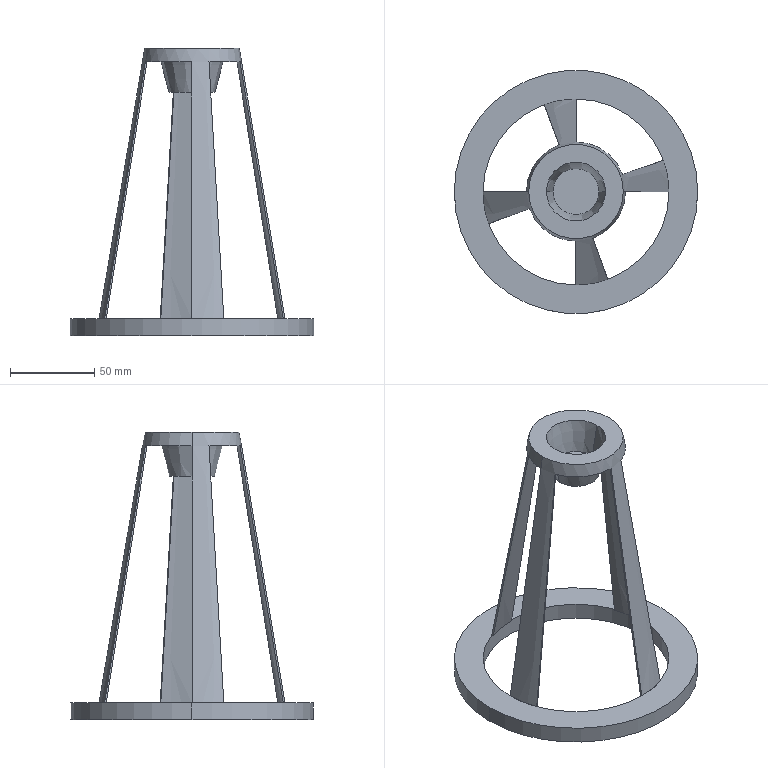Part | SolidWorks | features BaseBody 2 | 2 solids | 34 faces | box 144 x 144 x 170 mm | volume 89081 mm3 | plane 22 | cone 8 | cylinder 4 | commonest cylinder face diameters 110 x2 144 x2
STEP:
#1=CARTESIAN_POINT('',(55.,0.,0.));
#2=VERTEX_POINT('',#1);
#3=CARTESIAN_POINT('',(55.,0.,-10.));
#4=VERTEX_POINT('',#3);
#5=CARTESIAN_POINT('',(55.,0.,0.));
#6=DIRECTION('',(0.,0.,-1.));
#7=VECTOR('',#6,1000.);
#8=LINE('',#5,#7);
#9=EDGE_CURVE('',#2,#4,#8,.T.);
#10=ORIENTED_EDGE('',*,*,#9,.F.);
#11=CARTESIAN_POINT('',(-55.,0.,0.));
#12=VERTEX_POINT('',#11);
#13=CARTESIAN_POINT('',(0.,0.,0.));
#14=DIRECTION('',(0.,0.,-1.));
#15=DIRECTION('',(-1.,0.,0.));
#16=AXIS2_PLACEMENT_3D('',#13,#14,#15);
#17=CIRCLE('',#16,55.);
#18=EDGE_CURVE('',#12,#2,#17,.T.);
#19=ORIENTED_EDGE('',*,*,#18,.F.);
#20=CARTESIAN_POINT('',(-55.,0.,-10.));
#21=VERTEX_POINT('',#20);
#22=CARTESIAN_POINT('',(-55.,0.,0.));
#23=DIRECTION('',(0.,0.,-1.));
#24=VECTOR('',#23,1000.);
#25=LINE('',#22,#24);
#26=EDGE_CURVE('',#12,#21,#25,.T.);
#27=ORIENTED_EDGE('',*,*,#26,.T.);
#28=CARTESIAN_POINT('',(0.,0.,-10.));
#29=DIRECTION('',(0.,0.,-1.));
#30=DIRECTION('',(-1.,0.,0.));
#31=AXIS2_PLACEMENT_3D('',#28,#29,#30);
#32=CIRCLE('',#31,55.);
#33=EDGE_CURVE('',#21,#4,#32,.T.);
#34=ORIENTED_EDGE('',*,*,#33,.T.);
#35=EDGE_LOOP('',(#10,#19,#27,#34));
#36=FACE_OUTER_BOUND('',#35,.T.);
#37=CARTESIAN_POINT('',(0.,0.,0.));
#38=DIRECTION('',(0.,0.,-1.));
#39=DIRECTION('',(-1.,0.,0.));
#40=AXIS2_PLACEMENT_3D('',#37,#38,#39);
#41=CYLINDRICAL_SURFACE('',#40,55.);
#42=ADVANCED_FACE('',(#36),#41,.F.);
#43=ORIENTED_EDGE('',*,*,#33,.F.);
#44=CARTESIAN_POINT('',(0.,0.,-10.));
#45=DIRECTION('',(0.,0.,-1.));
#46=DIRECTION('',(-1.,0.,0.));
#47=AXIS2_PLACEMENT_3D('',#44,#45,#46);
#48=CIRCLE('',#47,55.);
#49=EDGE_CURVE('',#4,#21,#48,.T.);
#50=ORIENTED_EDGE('',*,*,#49,.F.);
#51=EDGE_LOOP('',(#43,#50));
#52=FACE_BOUND('',#51,.T.);
#53=CARTESIAN_POINT('',(72.,0.,-10.));
#54=VERTEX_POINT('',#53);
#55=CARTESIAN_POINT('',(-72.,0.,-10.));
#56=VERTEX_POINT('',#55);
#57=CARTESIAN_POINT('',(0.,0.,-10.));
#58=DIRECTION('',(0.,0.,-1.));
#59=DIRECTION('',(-1.,0.,0.));
#60=AXIS2_PLACEMENT_3D('',#57,#58,#59);
#61=CIRCLE('',#60,72.);
#62=EDGE_CURVE('',#54,#56,#61,.T.);
#63=ORIENTED_EDGE('',*,*,#62,.T.);
#64=CARTESIAN_POINT('',(0.,0.,-10.));
#65=DIRECTION('',(0.,0.,-1.));
#66=DIRECTION('',(-1.,0.,0.));
#67=AXIS2_PLACEMENT_3D('',#64,#65,#66);
#68=CIRCLE('',#67,72.);
#69=EDGE_CURVE('',#56,#54,#68,.T.);
#70=ORIENTED_EDGE('',*,*,#69,.T.);
#71=EDGE_LOOP('',(#63,#70));
#72=FACE_OUTER_BOUND('',#71,.T.);
#73=CARTESIAN_POINT('',(0.,0.,-10.));
#74=DIRECTION('',(0.,0.,-1.));
#75=DIRECTION('',(0.,-1.,0.));
#76=AXIS2_PLACEMENT_3D('',#73,#74,#75);
#77=PLANE('',#76);
#78=ADVANCED_FACE('',(#52,#72),#77,.T.);
#79=CARTESIAN_POINT('',(-72.,0.,0.));
#80=VERTEX_POINT('',#79);
#81=CARTESIAN_POINT('',(-72.,0.,-10.));
#82=DIRECTION('',(0.,0.,1.));
#83=VECTOR('',#82,1000.);
#84=LINE('',#81,#83);
#85=EDGE_CURVE('',#56,#80,#84,.T.);
#86=ORIENTED_EDGE('',*,*,#85,.F.);
#87=ORIENTED_EDGE('',*,*,#62,.F.);
#88=CARTESIAN_POINT('',(72.,0.,0.));
#89=VERTEX_POINT('',#88);
#90=CARTESIAN_POINT('',(72.,0.,-10.));
#91=DIRECTION('',(0.,0.,1.));
#92=VECTOR('',#91,1000.);
#93=LINE('',#90,#92);
#94=EDGE_CURVE('',#54,#89,#93,.T.);
#95=ORIENTED_EDGE('',*,*,#94,.T.);
#96=CARTESIAN_POINT('',(0.,0.,0.));
#97=DIRECTION('',(0.,0.,-1.));
#98=DIRECTION('',(-1.,0.,0.));
#99=AXIS2_PLACEMENT_3D('',#96,#97,#98);
#100=CIRCLE('',#99,72.);
#101=EDGE_CURVE('',#89,#80,#100,.T.);
#102=ORIENTED_EDGE('',*,*,#101,.T.);
#103=EDGE_LOOP('',(#86,#87,#95,#102));
#104=FACE_OUTER_BOUND('',#103,.T.);
#105=CARTESIAN_POINT('',(0.,0.,-10.));
#106=DIRECTION('',(0.,0.,1.));
#107=DIRECTION('',(1.,0.,0.));
#108=AXIS2_PLACEMENT_3D('',#105,#106,#107);
#109=CYLINDRICAL_SURFACE('',#108,72.);
#110=ADVANCED_FACE('',(#104),#109,.T.);
#111=ORIENTED_EDGE('',*,*,#18,.T.);
#112=CARTESIAN_POINT('',(0.,0.,0.));
#113=DIRECTION('',(0.,0.,-1.));
#114=DIRECTION('',(-1.,0.,0.));
#115=AXIS2_PLACEMENT_3D('',#112,#113,#114);
#116=CIRCLE('',#115,55.);
#117=EDGE_CURVE('',#2,#12,#116,.T.);
#118=ORIENTED_EDGE('',*,*,#117,.T.);
#119=EDGE_LOOP('',(#111,#118));
#120=FACE_BOUND('',#119,.T.);
#121=ORIENTED_EDGE('',*,*,#101,.F.);
#122=CARTESIAN_POINT('',(0.,0.,0.));
#123=DIRECTION('',(0.,0.,-1.));
#124=DIRECTION('',(-1.,0.,0.));
#125=AXIS2_PLACEMENT_3D('',#122,#123,#124);
#126=CIRCLE('',#125,72.);
#127=EDGE_CURVE('',#80,#89,#126,.T.);
#128=ORIENTED_EDGE('',*,*,#127,.F.);
#129=EDGE_LOOP('',(#121,#128));
#130=FACE_OUTER_BOUND('',#129,.T.);
#131=CARTESIAN_POINT('',(0.,0.,0.));
#132=DIRECTION('',(0.,0.,-1.));
#133=DIRECTION('',(0.,-1.,0.));
#134=AXIS2_PLACEMENT_3D('',#131,#132,#133);
#135=PLANE('',#134);
#136=ADVANCED_FACE('',(#120,#130),#135,.F.);
#137=ORIENTED_EDGE('',*,*,#69,.F.);
#138=ORIENTED_EDGE('',*,*,#85,.T.);
#139=ORIENTED_EDGE('',*,*,#127,.T.);
#140=ORIENTED_EDGE('',*,*,#94,.F.);
#141=EDGE_LOOP('',(#137,#138,#139,#140));
#142=FACE_OUTER_BOUND('',#141,.T.);
#143=CARTESIAN_POINT('',(0.,0.,-10.));
#144=DIRECTION('',(0.,0.,1.));
#145=DIRECTION('',(1.,0.,0.));
#146=AXIS2_PLACEMENT_3D('',#143,#144,#145);
#147=CYLINDRICAL_SURFACE('',#146,72.);
#148=ADVANCED_FACE('',(#142),#147,.T.);
#149=ORIENTED_EDGE('',*,*,#117,.F.);
#150=ORIENTED_EDGE('',*,*,#9,.T.);
#151=ORIENTED_EDGE('',*,*,#49,.T.);
#152=ORIENTED_EDGE('',*,*,#26,.F.);
#153=EDGE_LOOP('',(#149,#150,#151,#152));
#154=FACE_OUTER_BOUND('',#153,.T.);
#155=CARTESIAN_POINT('',(0.,0.,0.));
#156=DIRECTION('',(0.,0.,-1.));
#157=DIRECTION('',(-1.,0.,0.));
#158=AXIS2_PLACEMENT_3D('',#155,#156,#157);
#159=CYLINDRICAL_SURFACE('',#158,55.);
#160=ADVANCED_FACE('',(#154),#159,.F.);
#161=CLOSED_SHELL('',(#42,#78,#110,#136,#148,#160));
#162=MANIFOLD_SOLID_BREP('',#161);
#163=CARTESIAN_POINT('',(13.612,0.,140.));
#164=VERTEX_POINT('',#163);
#165=CARTESIAN_POINT('',(-13.612,0.,140.));
#166=VERTEX_POINT('',#165);
#167=CARTESIAN_POINT('',(0.,0.,140.));
#168=DIRECTION('',(0.,0.,1.));
#169=DIRECTION('',(1.,0.,0.));
#170=AXIS2_PLACEMENT_3D('',#167,#168,#169);
#171=CIRCLE('',#170,13.612);
#172=EDGE_CURVE('',#164,#166,#171,.T.);
#173=ORIENTED_EDGE('',*,*,#172,.T.);
#174=CARTESIAN_POINT('',(0.,0.,140.));
#175=DIRECTION('',(0.,0.,1.));
#176=DIRECTION('',(1.,0.,0.));
#177=AXIS2_PLACEMENT_3D('',#174,#175,#176);
#178=CIRCLE('',#177,13.612);
#179=EDGE_CURVE('',#166,#164,#178,.T.);
#180=ORIENTED_EDGE('',*,*,#179,.T.);
#181=EDGE_LOOP('',(#173,#180));
#182=FACE_OUTER_BOUND('',#181,.T.);
#183=CARTESIAN_POINT('',(0.,0.,140.));
#184=DIRECTION('',(0.,0.,1.));
#185=DIRECTION('',(1.,0.,0.));
#186=AXIS2_PLACEMENT_3D('',#183,#184,#185);
#187=PLANE('',#186);
#188=ADVANCED_FACE('',(#182),#187,.T.);
#189=CARTESIAN_POINT('',(-17.5,0.,160.));
#190=VERTEX_POINT('',#189);
#191=CARTESIAN_POINT('',(-17.5,0.,160.));
#192=DIRECTION('',(-0.1908,0.,0.9816));
#193=VECTOR('',#192,1000.);
#194=LINE('',#191,#193);
#195=EDGE_CURVE('',#166,#190,#194,.T.);
#196=ORIENTED_EDGE('',*,*,#195,.F.);
#197=ORIENTED_EDGE('',*,*,#172,.F.);
#198=CARTESIAN_POINT('',(17.5,0.,160.));
#199=VERTEX_POINT('',#198);
#200=CARTESIAN_POINT('',(17.5,0.,160.));
#201=DIRECTION('',(0.1908,0.,0.9816));
#202=VECTOR('',#201,1000.);
#203=LINE('',#200,#202);
#204=EDGE_CURVE('',#164,#199,#203,.T.);
#205=ORIENTED_EDGE('',*,*,#204,.T.);
#206=CARTESIAN_POINT('',(0.,0.,160.));
#207=DIRECTION('',(0.,0.,1.));
#208=DIRECTION('',(1.,0.,0.));
#209=AXIS2_PLACEMENT_3D('',#206,#207,#208);
#210=CIRCLE('',#209,17.5);
#211=EDGE_CURVE('',#199,#190,#210,.T.);
#212=ORIENTED_EDGE('',*,*,#211,.T.);
#213=EDGE_LOOP('',(#196,#197,#205,#212));
#214=FACE_OUTER_BOUND('',#213,.T.);
#215=CARTESIAN_POINT('',(0.,0.,160.));
#216=DIRECTION('',(0.,0.,1.));
#217=DIRECTION('',(1.,0.,0.));
#218=AXIS2_PLACEMENT_3D('',#215,#216,#217);
#219=CONICAL_SURFACE('',#218,17.5,0.192);
#220=ADVANCED_FACE('',(#214),#219,.F.);
#221=CARTESIAN_POINT('',(-13.569,0.,134.));
#222=VERTEX_POINT('',#221);
#223=CARTESIAN_POINT('',(13.569,0.,134.));
#224=VERTEX_POINT('',#223);
#225=CARTESIAN_POINT('',(0.,0.,134.));
#226=DIRECTION('',(0.,0.,-1.));
#227=DIRECTION('',(-1.,0.,0.));
#228=AXIS2_PLACEMENT_3D('',#225,#226,#227);
#229=CIRCLE('',#228,13.569);
#230=EDGE_CURVE('',#222,#224,#229,.T.);
#231=ORIENTED_EDGE('',*,*,#230,.T.);
#232=CARTESIAN_POINT('',(0.,0.,134.));
#233=DIRECTION('',(0.,0.,-1.));
#234=DIRECTION('',(-1.,0.,0.));
#235=AXIS2_PLACEMENT_3D('',#232,#233,#234);
#236=CIRCLE('',#235,13.569);
#237=EDGE_CURVE('',#224,#222,#236,.T.);
#238=ORIENTED_EDGE('',*,*,#237,.T.);
#239=EDGE_LOOP('',(#231,#238));
#240=FACE_OUTER_BOUND('',#239,.T.);
#241=CARTESIAN_POINT('',(0.,0.,134.));
#242=DIRECTION('',(0.,0.,-1.));
#243=DIRECTION('',(0.,-1.,0.));
#244=AXIS2_PLACEMENT_3D('',#241,#242,#243);
#245=PLANE('',#244);
#246=ADVANCED_FACE('',(#240),#245,.T.);
#247=CARTESIAN_POINT('',(20.,0.,158.));
#248=VERTEX_POINT('',#247);
#249=CARTESIAN_POINT('',(20.,0.,158.));
#250=DIRECTION('',(0.2588,0.,0.9659));
#251=VECTOR('',#250,1000.);
#252=LINE('',#249,#251);
#253=EDGE_CURVE('',#224,#248,#252,.T.);
#254=ORIENTED_EDGE('',*,*,#253,.F.);
#255=ORIENTED_EDGE('',*,*,#230,.F.);
#256=CARTESIAN_POINT('',(-20.,0.,158.));
#257=VERTEX_POINT('',#256);
#258=CARTESIAN_POINT('',(-20.,0.,158.));
#259=DIRECTION('',(-0.2588,0.,0.9659));
#260=VECTOR('',#259,1000.);
#261=LINE('',#258,#260);
#262=EDGE_CURVE('',#222,#257,#261,.T.);
#263=ORIENTED_EDGE('',*,*,#262,.T.);
#264=CARTESIAN_POINT('',(0.,0.,158.));
#265=DIRECTION('',(0.,0.,-1.));
#266=DIRECTION('',(1.,0.,0.));
#267=AXIS2_PLACEMENT_3D('',#264,#265,#266);
#268=CIRCLE('',#267,20.);
#269=EDGE_CURVE('',#257,#248,#268,.T.);
#270=ORIENTED_EDGE('',*,*,#269,.T.);
#271=EDGE_LOOP('',(#254,#255,#263,#270));
#272=FACE_OUTER_BOUND('',#271,.T.);
#273=CARTESIAN_POINT('',(0.,0.,158.));
#274=DIRECTION('',(0.,0.,1.));
#275=DIRECTION('',(-1.,0.,0.));
#276=AXIS2_PLACEMENT_3D('',#273,#274,#275);
#277=CONICAL_SURFACE('',#276,20.,0.2618);
#278=ADVANCED_FACE('',(#272),#277,.T.);
#279=CARTESIAN_POINT('',(0.,-28.336,152.));
#280=VERTEX_POINT('',#279);
#281=CARTESIAN_POINT('',(0.,-53.986,0.));
#282=VERTEX_POINT('',#281);
#283=CARTESIAN_POINT('',(0.,0.,319.916));
#284=DIRECTION('',(0.,-0.1664,-0.9861));
#285=VECTOR('',#284,1000.);
#286=LINE('',#283,#285);
#287=EDGE_CURVE('',#280,#282,#286,.T.);
#288=ORIENTED_EDGE('',*,*,#287,.T.);
#289=CARTESIAN_POINT('',(0.,-55.,0.));
#290=VERTEX_POINT('',#289);
#291=CARTESIAN_POINT('',(0.,-49.,0.));
#292=DIRECTION('',(0.,-1.,0.));
#293=VECTOR('',#292,1000.);
#294=LINE('',#291,#293);
#295=EDGE_CURVE('',#282,#290,#294,.T.);
#296=ORIENTED_EDGE('',*,*,#295,.T.);
#297=CARTESIAN_POINT('',(0.,-29.35,152.));
#298=VERTEX_POINT('',#297);
#299=CARTESIAN_POINT('',(0.,-55.,0.));
#300=DIRECTION('',(0.,0.1664,0.9861));
#301=VECTOR('',#300,1000.);
#302=LINE('',#299,#301);
#303=EDGE_CURVE('',#290,#298,#302,.T.);
#304=ORIENTED_EDGE('',*,*,#303,.T.);
#305=CARTESIAN_POINT('',(0.,-29.35,152.));
#306=DIRECTION('',(0.,1.,0.));
#307=VECTOR('',#306,1000.);
#308=LINE('',#305,#307);
#309=EDGE_CURVE('',#298,#280,#308,.T.);
#310=ORIENTED_EDGE('',*,*,#309,.T.);
#311=EDGE_LOOP('',(#288,#296,#304,#310));
#312=FACE_OUTER_BOUND('',#311,.T.);
#313=CARTESIAN_POINT('',(0.,0.,0.));
#314=DIRECTION('',(-1.,0.,0.));
#315=DIRECTION('',(0.,0.,1.));
#316=AXIS2_PLACEMENT_3D('',#313,#314,#315);
#317=PLANE('',#316);
#318=ADVANCED_FACE('',(#312),#317,.T.);
#319=CARTESIAN_POINT('',(-27.58,-10.038,152.));
#320=VERTEX_POINT('',#319);
#321=CARTESIAN_POINT('',(-26.627,-9.691,152.));
#322=VERTEX_POINT('',#321);
#323=CARTESIAN_POINT('',(-27.58,-10.038,152.));
#324=DIRECTION('',(0.9397,0.342,0.));
#325=VECTOR('',#324,1000.);
#326=LINE('',#323,#325);
#327=EDGE_CURVE('',#320,#322,#326,.T.);
#328=ORIENTED_EDGE('',*,*,#327,.F.);
#329=CARTESIAN_POINT('',(-51.683,-18.811,0.));
#330=VERTEX_POINT('',#329);
#331=CARTESIAN_POINT('',(-51.683,-18.811,0.));
#332=DIRECTION('',(0.1564,0.05691,0.9861));
#333=VECTOR('',#332,1000.);
#334=LINE('',#331,#333);
#335=EDGE_CURVE('',#330,#320,#334,.T.);
#336=ORIENTED_EDGE('',*,*,#335,.F.);
#337=CARTESIAN_POINT('',(-50.73,-18.464,0.));
#338=VERTEX_POINT('',#337);
#339=CARTESIAN_POINT('',(-46.045,-16.759,0.));
#340=DIRECTION('',(-0.9397,-0.342,0.));
#341=VECTOR('',#340,1000.);
#342=LINE('',#339,#341);
#343=EDGE_CURVE('',#338,#330,#342,.T.);
#344=ORIENTED_EDGE('',*,*,#343,.F.);
#345=CARTESIAN_POINT('',(0.,0.,319.916));
#346=DIRECTION('',(-0.1564,-0.05691,-0.9861));
#347=VECTOR('',#346,1000.);
#348=LINE('',#345,#347);
#349=EDGE_CURVE('',#322,#338,#348,.T.);
#350=ORIENTED_EDGE('',*,*,#349,.F.);
#351=EDGE_LOOP('',(#328,#336,#344,#350));
#352=FACE_OUTER_BOUND('',#351,.T.);
#353=CARTESIAN_POINT('',(0.,0.,0.));
#354=DIRECTION('',(-0.342,0.9397,0.));
#355=DIRECTION('',(0.,0.,1.));
#356=AXIS2_PLACEMENT_3D('',#353,#354,#355);
#357=PLANE('',#356);
#358=ADVANCED_FACE('',(#352),#357,.F.);
#359=CARTESIAN_POINT('',(0.,0.,152.));
#360=DIRECTION('',(0.,0.,1.));
#361=DIRECTION('',(-1.,0.,0.));
#362=AXIS2_PLACEMENT_3D('',#359,#360,#361);
#363=CIRCLE('',#362,28.336);
#364=EDGE_CURVE('',#322,#280,#363,.T.);
#365=ORIENTED_EDGE('',*,*,#364,.T.);
#366=ORIENTED_EDGE('',*,*,#309,.F.);
#367=CARTESIAN_POINT('',(0.,0.,152.));
#368=DIRECTION('',(0.,0.,1.));
#369=DIRECTION('',(0.,1.,0.));
#370=AXIS2_PLACEMENT_3D('',#367,#368,#369);
#371=CIRCLE('',#370,29.35);
#372=EDGE_CURVE('',#320,#298,#371,.T.);
#373=ORIENTED_EDGE('',*,*,#372,.F.);
#374=ORIENTED_EDGE('',*,*,#327,.T.);
#375=EDGE_LOOP('',(#365,#366,#373,#374));
#376=FACE_OUTER_BOUND('',#375,.T.);
#377=CARTESIAN_POINT('',(-27.58,-10.038,152.));
#378=DIRECTION('',(0.,0.,-1.));
#379=DIRECTION('',(0.,-1.,0.));
#380=AXIS2_PLACEMENT_3D('',#377,#378,#379);
#381=PLANE('',#380);
#382=ADVANCED_FACE('',(#376),#381,.T.);
#383=CARTESIAN_POINT('',(28.336,0.,152.));
#384=VERTEX_POINT('',#383);
#385=CARTESIAN_POINT('',(53.986,0.,0.));
#386=VERTEX_POINT('',#385);
#387=CARTESIAN_POINT('',(0.,0.,319.916));
#388=DIRECTION('',(0.1664,0.,-0.9861));
#389=VECTOR('',#388,1000.);
#390=LINE('',#387,#389);
#391=EDGE_CURVE('',#384,#386,#390,.T.);
#392=ORIENTED_EDGE('',*,*,#391,.T.);
#393=CARTESIAN_POINT('',(55.,0.,0.));
#394=VERTEX_POINT('',#393);
#395=CARTESIAN_POINT('',(49.,0.,0.));
#396=DIRECTION('',(1.,0.,0.));
#397=VECTOR('',#396,1000.);
#398=LINE('',#395,#397);
#399=EDGE_CURVE('',#386,#394,#398,.T.);
#400=ORIENTED_EDGE('',*,*,#399,.T.);
#401=CARTESIAN_POINT('',(29.35,0.,152.));
#402=VERTEX_POINT('',#401);
#403=CARTESIAN_POINT('',(55.,0.,0.));
#404=DIRECTION('',(-0.1664,0.,0.9861));
#405=VECTOR('',#404,1000.);
#406=LINE('',#403,#405);
#407=EDGE_CURVE('',#394,#402,#406,.T.);
#408=ORIENTED_EDGE('',*,*,#407,.T.);
#409=CARTESIAN_POINT('',(29.35,0.,152.));
#410=DIRECTION('',(-1.,0.,0.));
#411=VECTOR('',#410,1000.);
#412=LINE('',#409,#411);
#413=EDGE_CURVE('',#402,#384,#412,.T.);
#414=ORIENTED_EDGE('',*,*,#413,.T.);
#415=EDGE_LOOP('',(#392,#400,#408,#414));
#416=FACE_OUTER_BOUND('',#415,.T.);
#417=CARTESIAN_POINT('',(0.,0.,0.));
#418=DIRECTION('',(0.,-1.,0.));
#419=DIRECTION('',(0.,0.,-1.));
#420=AXIS2_PLACEMENT_3D('',#417,#418,#419);
#421=PLANE('',#420);
#422=ADVANCED_FACE('',(#416),#421,.T.);
#423=CARTESIAN_POINT('',(10.038,-27.58,152.));
#424=VERTEX_POINT('',#423);
#425=CARTESIAN_POINT('',(9.691,-26.627,152.));
#426=VERTEX_POINT('',#425);
#427=CARTESIAN_POINT('',(10.038,-27.58,152.));
#428=DIRECTION('',(-0.342,0.9397,0.));
#429=VECTOR('',#428,1000.);
#430=LINE('',#427,#429);
#431=EDGE_CURVE('',#424,#426,#430,.T.);
#432=ORIENTED_EDGE('',*,*,#431,.F.);
#433=CARTESIAN_POINT('',(18.811,-51.683,0.));
#434=VERTEX_POINT('',#433);
#435=CARTESIAN_POINT('',(18.811,-51.683,0.));
#436=DIRECTION('',(-0.05691,0.1564,0.9861));
#437=VECTOR('',#436,1000.);
#438=LINE('',#435,#437);
#439=EDGE_CURVE('',#434,#424,#438,.T.);
#440=ORIENTED_EDGE('',*,*,#439,.F.);
#441=CARTESIAN_POINT('',(18.464,-50.73,0.));
#442=VERTEX_POINT('',#441);
#443=CARTESIAN_POINT('',(16.759,-46.045,0.));
#444=DIRECTION('',(0.342,-0.9397,0.));
#445=VECTOR('',#444,1000.);
#446=LINE('',#443,#445);
#447=EDGE_CURVE('',#442,#434,#446,.T.);
#448=ORIENTED_EDGE('',*,*,#447,.F.);
#449=CARTESIAN_POINT('',(0.,0.,319.916));
#450=DIRECTION('',(0.05691,-0.1564,-0.9861));
#451=VECTOR('',#450,1000.);
#452=LINE('',#449,#451);
#453=EDGE_CURVE('',#426,#442,#452,.T.);
#454=ORIENTED_EDGE('',*,*,#453,.F.);
#455=EDGE_LOOP('',(#432,#440,#448,#454));
#456=FACE_OUTER_BOUND('',#455,.T.);
#457=CARTESIAN_POINT('',(0.,0.,0.));
#458=DIRECTION('',(-0.9397,-0.342,0.));
#459=DIRECTION('',(-0.342,0.9397,0.));
#460=AXIS2_PLACEMENT_3D('',#457,#458,#459);
#461=PLANE('',#460);
#462=ADVANCED_FACE('',(#456),#461,.F.);
#463=CARTESIAN_POINT('',(0.,0.,152.));
#464=DIRECTION('',(0.,0.,1.));
#465=DIRECTION('',(-1.,0.,0.));
#466=AXIS2_PLACEMENT_3D('',#463,#464,#465);
#467=CIRCLE('',#466,28.336);
#468=EDGE_CURVE('',#426,#384,#467,.T.);
#469=ORIENTED_EDGE('',*,*,#468,.T.);
#470=ORIENTED_EDGE('',*,*,#413,.F.);
#471=CARTESIAN_POINT('',(0.,0.,152.));
#472=DIRECTION('',(0.,0.,1.));
#473=DIRECTION('',(-1.,0.,0.));
#474=AXIS2_PLACEMENT_3D('',#471,#472,#473);
#475=CIRCLE('',#474,29.35);
#476=EDGE_CURVE('',#424,#402,#475,.T.);
#477=ORIENTED_EDGE('',*,*,#476,.F.);
#478=ORIENTED_EDGE('',*,*,#431,.T.);
#479=EDGE_LOOP('',(#469,#470,#477,#478));
#480=FACE_OUTER_BOUND('',#479,.T.);
#481=CARTESIAN_POINT('',(10.038,-27.58,152.));
#482=DIRECTION('',(0.,0.,-1.));
#483=DIRECTION('',(0.,-1.,0.));
#484=AXIS2_PLACEMENT_3D('',#481,#482,#483);
#485=PLANE('',#484);
#486=ADVANCED_FACE('',(#480),#485,.T.);
#487=CARTESIAN_POINT('',(0.,28.336,152.));
#488=VERTEX_POINT('',#487);
#489=CARTESIAN_POINT('',(0.,53.986,0.));
#490=VERTEX_POINT('',#489);
#491=CARTESIAN_POINT('',(0.,0.,319.916));
#492=DIRECTION('',(0.,0.1664,-0.9861));
#493=VECTOR('',#492,1000.);
#494=LINE('',#491,#493);
#495=EDGE_CURVE('',#488,#490,#494,.T.);
#496=ORIENTED_EDGE('',*,*,#495,.T.);
#497=CARTESIAN_POINT('',(0.,55.,0.));
#498=VERTEX_POINT('',#497);
#499=CARTESIAN_POINT('',(0.,49.,0.));
#500=DIRECTION('',(0.,1.,0.));
#501=VECTOR('',#500,1000.);
#502=LINE('',#499,#501);
#503=EDGE_CURVE('',#490,#498,#502,.T.);
#504=ORIENTED_EDGE('',*,*,#503,.T.);
#505=CARTESIAN_POINT('',(0.,29.35,152.));
#506=VERTEX_POINT('',#505);
#507=CARTESIAN_POINT('',(0.,55.,0.));
#508=DIRECTION('',(0.,-0.1664,0.9861));
#509=VECTOR('',#508,1000.);
#510=LINE('',#507,#509);
#511=EDGE_CURVE('',#498,#506,#510,.T.);
#512=ORIENTED_EDGE('',*,*,#511,.T.);
#513=CARTESIAN_POINT('',(0.,29.35,152.));
#514=DIRECTION('',(0.,-1.,0.));
#515=VECTOR('',#514,1000.);
#516=LINE('',#513,#515);
#517=EDGE_CURVE('',#506,#488,#516,.T.);
#518=ORIENTED_EDGE('',*,*,#517,.T.);
#519=EDGE_LOOP('',(#496,#504,#512,#518));
#520=FACE_OUTER_BOUND('',#519,.T.);
#521=CARTESIAN_POINT('',(0.,0.,0.));
#522=DIRECTION('',(1.,0.,0.));
#523=DIRECTION('',(0.,-1.,0.));
#524=AXIS2_PLACEMENT_3D('',#521,#522,#523);
#525=PLANE('',#524);
#526=ADVANCED_FACE('',(#520),#525,.T.);
#527=CARTESIAN_POINT('',(27.58,10.038,152.));
#528=VERTEX_POINT('',#527);
#529=CARTESIAN_POINT('',(26.627,9.691,152.));
#530=VERTEX_POINT('',#529);
#531=CARTESIAN_POINT('',(27.58,10.038,152.));
#532=DIRECTION('',(-0.9397,-0.342,0.));
#533=VECTOR('',#532,1000.);
#534=LINE('',#531,#533);
#535=EDGE_CURVE('',#528,#530,#534,.T.);
#536=ORIENTED_EDGE('',*,*,#535,.F.);
#537=CARTESIAN_POINT('',(51.683,18.811,0.));
#538=VERTEX_POINT('',#537);
#539=CARTESIAN_POINT('',(51.683,18.811,0.));
#540=DIRECTION('',(-0.1564,-0.05691,0.9861));
#541=VECTOR('',#540,1000.);
#542=LINE('',#539,#541);
#543=EDGE_CURVE('',#538,#528,#542,.T.);
#544=ORIENTED_EDGE('',*,*,#543,.F.);
#545=CARTESIAN_POINT('',(50.73,18.464,0.));
#546=VERTEX_POINT('',#545);
#547=CARTESIAN_POINT('',(46.045,16.759,0.));
#548=DIRECTION('',(0.9397,0.342,0.));
#549=VECTOR('',#548,1000.);
#550=LINE('',#547,#549);
#551=EDGE_CURVE('',#546,#538,#550,.T.);
#552=ORIENTED_EDGE('',*,*,#551,.F.);
#553=CARTESIAN_POINT('',(0.,0.,319.916));
#554=DIRECTION('',(0.1564,0.05691,-0.9861));
#555=VECTOR('',#554,1000.);
#556=LINE('',#553,#555);
#557=EDGE_CURVE('',#530,#546,#556,.T.);
#558=ORIENTED_EDGE('',*,*,#557,.F.);
#559=EDGE_LOOP('',(#536,#544,#552,#558));
#560=FACE_OUTER_BOUND('',#559,.T.);
#561=CARTESIAN_POINT('',(0.,0.,0.));
#562=DIRECTION('',(0.342,-0.9397,0.));
#563=DIRECTION('',(0.,0.,-1.));
#564=AXIS2_PLACEMENT_3D('',#561,#562,#563);
#565=PLANE('',#564);
#566=ADVANCED_FACE('',(#560),#565,.F.);
#567=CARTESIAN_POINT('',(0.,0.,152.));
#568=DIRECTION('',(0.,0.,1.));
#569=DIRECTION('',(-1.,0.,0.));
#570=AXIS2_PLACEMENT_3D('',#567,#568,#569);
#571=CIRCLE('',#570,28.336);
#572=EDGE_CURVE('',#530,#488,#571,.T.);
#573=ORIENTED_EDGE('',*,*,#572,.T.);
#574=ORIENTED_EDGE('',*,*,#517,.F.);
#575=CARTESIAN_POINT('',(0.,0.,152.));
#576=DIRECTION('',(0.,0.,1.));
#577=DIRECTION('',(0.,-1.,0.));
#578=AXIS2_PLACEMENT_3D('',#575,#576,#577);
#579=CIRCLE('',#578,29.35);
#580=EDGE_CURVE('',#528,#506,#579,.T.);
#581=ORIENTED_EDGE('',*,*,#580,.F.);
#582=ORIENTED_EDGE('',*,*,#535,.T.);
#583=EDGE_LOOP('',(#573,#574,#581,#582));
#584=FACE_OUTER_BOUND('',#583,.T.);
#585=CARTESIAN_POINT('',(27.58,10.038,152.));
#586=DIRECTION('',(0.,0.,-1.));
#587=DIRECTION('',(0.,-1.,0.));
#588=AXIS2_PLACEMENT_3D('',#585,#586,#587);
#589=PLANE('',#588);
#590=ADVANCED_FACE('',(#584),#589,.T.);
#591=CARTESIAN_POINT('',(-28.336,0.,152.));
#592=VERTEX_POINT('',#591);
#593=CARTESIAN_POINT('',(-53.986,0.,0.));
#594=VERTEX_POINT('',#593);
#595=CARTESIAN_POINT('',(0.,0.,319.916));
#596=DIRECTION('',(-0.1664,0.,-0.9861));
#597=VECTOR('',#596,1000.);
#598=LINE('',#595,#597);
#599=EDGE_CURVE('',#592,#594,#598,.T.);
#600=ORIENTED_EDGE('',*,*,#599,.T.);
#601=CARTESIAN_POINT('',(-55.,0.,0.));
#602=VERTEX_POINT('',#601);
#603=CARTESIAN_POINT('',(-49.,0.,0.));
#604=DIRECTION('',(-1.,0.,0.));
#605=VECTOR('',#604,1000.);
#606=LINE('',#603,#605);
#607=EDGE_CURVE('',#594,#602,#606,.T.);
#608=ORIENTED_EDGE('',*,*,#607,.T.);
#609=CARTESIAN_POINT('',(-29.35,0.,152.));
#610=VERTEX_POINT('',#609);
#611=CARTESIAN_POINT('',(-55.,0.,0.));
#612=DIRECTION('',(0.1664,0.,0.9861));
#613=VECTOR('',#612,1000.);
#614=LINE('',#611,#613);
#615=EDGE_CURVE('',#602,#610,#614,.T.);
#616=ORIENTED_EDGE('',*,*,#615,.T.);
#617=CARTESIAN_POINT('',(-29.35,0.,152.));
#618=DIRECTION('',(1.,0.,0.));
#619=VECTOR('',#618,1000.);
#620=LINE('',#617,#619);
#621=EDGE_CURVE('',#610,#592,#620,.T.);
#622=ORIENTED_EDGE('',*,*,#621,.T.);
#623=EDGE_LOOP('',(#600,#608,#616,#622));
#624=FACE_OUTER_BOUND('',#623,.T.);
#625=CARTESIAN_POINT('',(0.,0.,0.));
#626=DIRECTION('',(0.,1.,0.));
#627=DIRECTION('',(1.,0.,0.));
#628=AXIS2_PLACEMENT_3D('',#625,#626,#627);
#629=PLANE('',#628);
#630=ADVANCED_FACE('',(#624),#629,.T.);
#631=CARTESIAN_POINT('',(-10.038,27.58,152.));
#632=VERTEX_POINT('',#631);
#633=CARTESIAN_POINT('',(-9.691,26.627,152.));
#634=VERTEX_POINT('',#633);
#635=CARTESIAN_POINT('',(-10.038,27.58,152.));
#636=DIRECTION('',(0.342,-0.9397,0.));
#637=VECTOR('',#636,1000.);
#638=LINE('',#635,#637);
#639=EDGE_CURVE('',#632,#634,#638,.T.);
#640=ORIENTED_EDGE('',*,*,#639,.F.);
#641=CARTESIAN_POINT('',(-18.811,51.683,0.));
#642=VERTEX_POINT('',#641);
#643=CARTESIAN_POINT('',(-18.811,51.683,0.));
#644=DIRECTION('',(0.05691,-0.1564,0.9861));
#645=VECTOR('',#644,1000.);
#646=LINE('',#643,#645);
#647=EDGE_CURVE('',#642,#632,#646,.T.);
#648=ORIENTED_EDGE('',*,*,#647,.F.);
#649=CARTESIAN_POINT('',(-18.464,50.73,0.));
#650=VERTEX_POINT('',#649);
#651=CARTESIAN_POINT('',(-16.759,46.045,0.));
#652=DIRECTION('',(-0.342,0.9397,0.));
#653=VECTOR('',#652,1000.);
#654=LINE('',#651,#653);
#655=EDGE_CURVE('',#650,#642,#654,.T.);
#656=ORIENTED_EDGE('',*,*,#655,.F.);
#657=CARTESIAN_POINT('',(0.,0.,319.916));
#658=DIRECTION('',(-0.05691,0.1564,-0.9861));
#659=VECTOR('',#658,1000.);
#660=LINE('',#657,#659);
#661=EDGE_CURVE('',#634,#650,#660,.T.);
#662=ORIENTED_EDGE('',*,*,#661,.F.);
#663=EDGE_LOOP('',(#640,#648,#656,#662));
#664=FACE_OUTER_BOUND('',#663,.T.);
#665=CARTESIAN_POINT('',(0.,0.,0.));
#666=DIRECTION('',(0.9397,0.342,0.));
#667=DIRECTION('',(0.,0.,-1.));
#668=AXIS2_PLACEMENT_3D('',#665,#666,#667);
#669=PLANE('',#668);
#670=ADVANCED_FACE('',(#664),#669,.F.);
#671=CARTESIAN_POINT('',(0.,0.,152.));
#672=DIRECTION('',(0.,0.,1.));
#673=DIRECTION('',(-1.,0.,0.));
#674=AXIS2_PLACEMENT_3D('',#671,#672,#673);
#675=CIRCLE('',#674,28.336);
#676=EDGE_CURVE('',#634,#592,#675,.T.);
#677=ORIENTED_EDGE('',*,*,#676,.T.);
#678=ORIENTED_EDGE('',*,*,#621,.F.);
#679=CARTESIAN_POINT('',(0.,0.,152.));
#680=DIRECTION('',(0.,0.,1.));
#681=DIRECTION('',(1.,0.,0.));
#682=AXIS2_PLACEMENT_3D('',#679,#680,#681);
#683=CIRCLE('',#682,29.35);
#684=EDGE_CURVE('',#632,#610,#683,.T.);
#685=ORIENTED_EDGE('',*,*,#684,.F.);
#686=ORIENTED_EDGE('',*,*,#639,.T.);
#687=EDGE_LOOP('',(#677,#678,#685,#686));
#688=FACE_OUTER_BOUND('',#687,.T.);
#689=CARTESIAN_POINT('',(-10.038,27.58,152.));
#690=DIRECTION('',(0.,0.,-1.));
#691=DIRECTION('',(0.,-1.,0.));
#692=AXIS2_PLACEMENT_3D('',#689,#690,#691);
#693=PLANE('',#692);
#694=ADVANCED_FACE('',(#688),#693,.T.);
#695=CARTESIAN_POINT('',(28.,0.,160.));
#696=VERTEX_POINT('',#695);
#697=CARTESIAN_POINT('',(28.,0.,160.));
#698=DIRECTION('',(0.1664,0.,-0.9861));
#699=VECTOR('',#698,1000.);
#700=LINE('',#697,#699);
#701=EDGE_CURVE('',#696,#402,#700,.T.);
#702=ORIENTED_EDGE('',*,*,#701,.F.);
#703=CARTESIAN_POINT('',(-28.,0.,160.));
#704=VERTEX_POINT('',#703);
#705=CARTESIAN_POINT('',(0.,0.,160.));
#706=DIRECTION('',(0.,0.,1.));
#707=DIRECTION('',(1.,0.,0.));
#708=AXIS2_PLACEMENT_3D('',#705,#706,#707);
#709=CIRCLE('',#708,28.);
#710=EDGE_CURVE('',#704,#696,#709,.T.);
#711=ORIENTED_EDGE('',*,*,#710,.F.);
#712=CARTESIAN_POINT('',(-28.,0.,160.));
#713=DIRECTION('',(-0.1664,0.,-0.9861));
#714=VECTOR('',#713,1000.);
#715=LINE('',#712,#714);
#716=EDGE_CURVE('',#704,#610,#715,.T.);
#717=ORIENTED_EDGE('',*,*,#716,.T.);
#718=ORIENTED_EDGE('',*,*,#615,.F.);
#719=CARTESIAN_POINT('',(0.,0.,0.));
#720=DIRECTION('',(0.,0.,-1.));
#721=DIRECTION('',(-1.,0.,0.));
#722=AXIS2_PLACEMENT_3D('',#719,#720,#721);
#723=CIRCLE('',#722,55.);
#724=EDGE_CURVE('',#330,#602,#723,.T.);
#725=ORIENTED_EDGE('',*,*,#724,.F.);
#726=ORIENTED_EDGE('',*,*,#335,.T.);
#727=ORIENTED_EDGE('',*,*,#372,.T.);
#728=ORIENTED_EDGE('',*,*,#303,.F.);
#729=CARTESIAN_POINT('',(0.,0.,0.));
#730=DIRECTION('',(0.,0.,-1.));
#731=DIRECTION('',(-1.,0.,0.));
#732=AXIS2_PLACEMENT_3D('',#729,#730,#731);
#733=CIRCLE('',#732,55.);
#734=EDGE_CURVE('',#434,#290,#733,.T.);
#735=ORIENTED_EDGE('',*,*,#734,.F.);
#736=ORIENTED_EDGE('',*,*,#439,.T.);
#737=ORIENTED_EDGE('',*,*,#476,.T.);
#738=EDGE_LOOP('',(#702,#711,#717,#718,#725,#726,#727,#728,#735,#736,#737));
#739=FACE_OUTER_BOUND('',#738,.T.);
#740=CARTESIAN_POINT('',(0.,0.,160.));
#741=DIRECTION('',(0.,0.,-1.));
#742=DIRECTION('',(-1.,0.,0.));
#743=AXIS2_PLACEMENT_3D('',#740,#741,#742);
#744=CONICAL_SURFACE('',#743,28.,0.1672);
#745=ADVANCED_FACE('',(#739),#744,.T.);
#746=ORIENTED_EDGE('',*,*,#211,.F.);
#747=CARTESIAN_POINT('',(0.,0.,160.));
#748=DIRECTION('',(0.,0.,1.));
#749=DIRECTION('',(1.,0.,0.));
#750=AXIS2_PLACEMENT_3D('',#747,#748,#749);
#751=CIRCLE('',#750,17.5);
#752=EDGE_CURVE('',#190,#199,#751,.T.);
#753=ORIENTED_EDGE('',*,*,#752,.F.);
#754=EDGE_LOOP('',(#746,#753));
#755=FACE_BOUND('',#754,.T.);
#756=ORIENTED_EDGE('',*,*,#710,.T.);
#757=CARTESIAN_POINT('',(0.,0.,160.));
#758=DIRECTION('',(0.,0.,1.));
#759=DIRECTION('',(1.,0.,0.));
#760=AXIS2_PLACEMENT_3D('',#757,#758,#759);
#761=CIRCLE('',#760,28.);
#762=EDGE_CURVE('',#696,#704,#761,.T.);
#763=ORIENTED_EDGE('',*,*,#762,.T.);
#764=EDGE_LOOP('',(#756,#763));
#765=FACE_OUTER_BOUND('',#764,.T.);
#766=CARTESIAN_POINT('',(0.,0.,160.));
#767=DIRECTION('',(0.,0.,1.));
#768=DIRECTION('',(1.,0.,0.));
#769=AXIS2_PLACEMENT_3D('',#766,#767,#768);
#770=PLANE('',#769);
#771=ADVANCED_FACE('',(#755,#765),#770,.T.);
#772=ORIENTED_EDGE('',*,*,#343,.T.);
#773=ORIENTED_EDGE('',*,*,#724,.T.);
#774=ORIENTED_EDGE('',*,*,#607,.F.);
#775=CARTESIAN_POINT('',(0.,0.,0.));
#776=DIRECTION('',(0.,0.,1.));
#777=DIRECTION('',(1.,0.,0.));
#778=AXIS2_PLACEMENT_3D('',#775,#776,#777);
#779=CIRCLE('',#778,53.986);
#780=EDGE_CURVE('',#594,#338,#779,.T.);
#781=ORIENTED_EDGE('',*,*,#780,.T.);
#782=EDGE_LOOP('',(#772,#773,#774,#781));
#783=FACE_OUTER_BOUND('',#782,.T.);
#784=CARTESIAN_POINT('',(0.,0.,0.));
#785=DIRECTION('',(0.,0.,-1.));
#786=DIRECTION('',(0.,-1.,0.));
#787=AXIS2_PLACEMENT_3D('',#784,#785,#786);
#788=PLANE('',#787);
#789=ADVANCED_FACE('',(#783),#788,.T.);
#790=CARTESIAN_POINT('',(27.323,0.,158.));
#791=VERTEX_POINT('',#790);
#792=CARTESIAN_POINT('',(27.014,0.,159.834));
#793=DIRECTION('',(0.1664,0.,-0.9861));
#794=VECTOR('',#793,1000.);
#795=LINE('',#792,#794);
#796=EDGE_CURVE('',#791,#384,#795,.T.);
#797=ORIENTED_EDGE('',*,*,#796,.F.);
#798=CARTESIAN_POINT('',(-27.323,0.,158.));
#799=VERTEX_POINT('',#798);
#800=CARTESIAN_POINT('',(0.,0.,158.));
#801=DIRECTION('',(0.,0.,1.));
#802=DIRECTION('',(1.,0.,0.));
#803=AXIS2_PLACEMENT_3D('',#800,#801,#802);
#804=CIRCLE('',#803,27.323);
#805=EDGE_CURVE('',#791,#799,#804,.T.);
#806=ORIENTED_EDGE('',*,*,#805,.T.);
#807=CARTESIAN_POINT('',(-27.014,0.,159.834));
#808=DIRECTION('',(-0.1664,0.,-0.9861));
#809=VECTOR('',#808,1000.);
#810=LINE('',#807,#809);
#811=EDGE_CURVE('',#799,#592,#810,.T.);
#812=ORIENTED_EDGE('',*,*,#811,.T.);
#813=ORIENTED_EDGE('',*,*,#676,.F.);
#814=ORIENTED_EDGE('',*,*,#661,.T.);
#815=CARTESIAN_POINT('',(0.,0.,0.));
#816=DIRECTION('',(0.,0.,1.));
#817=DIRECTION('',(1.,0.,0.));
#818=AXIS2_PLACEMENT_3D('',#815,#816,#817);
#819=CIRCLE('',#818,53.986);
#820=EDGE_CURVE('',#490,#650,#819,.T.);
#821=ORIENTED_EDGE('',*,*,#820,.F.);
#822=ORIENTED_EDGE('',*,*,#495,.F.);
#823=ORIENTED_EDGE('',*,*,#572,.F.);
#824=ORIENTED_EDGE('',*,*,#557,.T.);
#825=CARTESIAN_POINT('',(0.,0.,0.));
#826=DIRECTION('',(0.,0.,1.));
#827=DIRECTION('',(1.,0.,0.));
#828=AXIS2_PLACEMENT_3D('',#825,#826,#827);
#829=CIRCLE('',#828,53.986);
#830=EDGE_CURVE('',#386,#546,#829,.T.);
#831=ORIENTED_EDGE('',*,*,#830,.F.);
#832=ORIENTED_EDGE('',*,*,#391,.F.);
#833=EDGE_LOOP('',(#797,#806,#812,#813,#814,#821,#822,#823,#824,#831,#832));
#834=FACE_OUTER_BOUND('',#833,.T.);
#835=CARTESIAN_POINT('',(0.,0.,159.834));
#836=DIRECTION('',(0.,0.,-1.));
#837=DIRECTION('',(-1.,0.,0.));
#838=AXIS2_PLACEMENT_3D('',#835,#836,#837);
#839=CONICAL_SURFACE('',#838,27.014,0.1672);
#840=ADVANCED_FACE('',(#834),#839,.F.);
#841=ORIENTED_EDGE('',*,*,#269,.F.);
#842=CARTESIAN_POINT('',(0.,0.,158.));
#843=DIRECTION('',(0.,0.,-1.));
#844=DIRECTION('',(1.,0.,0.));
#845=AXIS2_PLACEMENT_3D('',#842,#843,#844);
#846=CIRCLE('',#845,20.);
#847=EDGE_CURVE('',#248,#257,#846,.T.);
#848=ORIENTED_EDGE('',*,*,#847,.F.);
#849=EDGE_LOOP('',(#841,#848));
#850=FACE_BOUND('',#849,.T.);
#851=CARTESIAN_POINT('',(0.,0.,158.));
#852=DIRECTION('',(0.,0.,1.));
#853=DIRECTION('',(1.,0.,0.));
#854=AXIS2_PLACEMENT_3D('',#851,#852,#853);
#855=CIRCLE('',#854,27.323);
#856=EDGE_CURVE('',#799,#791,#855,.T.);
#857=ORIENTED_EDGE('',*,*,#856,.F.);
#858=ORIENTED_EDGE('',*,*,#805,.F.);
#859=EDGE_LOOP('',(#857,#858));
#860=FACE_OUTER_BOUND('',#859,.T.);
#861=CARTESIAN_POINT('',(0.,0.,158.));
#862=DIRECTION('',(0.,0.,1.));
#863=DIRECTION('',(1.,0.,0.));
#864=AXIS2_PLACEMENT_3D('',#861,#862,#863);
#865=PLANE('',#864);
#866=ADVANCED_FACE('',(#850,#860),#865,.F.);
#867=CARTESIAN_POINT('',(0.,0.,0.));
#868=DIRECTION('',(0.,0.,-1.));
#869=DIRECTION('',(-1.,0.,0.));
#870=AXIS2_PLACEMENT_3D('',#867,#868,#869);
#871=CIRCLE('',#870,55.);
#872=EDGE_CURVE('',#642,#498,#871,.T.);
#873=ORIENTED_EDGE('',*,*,#872,.T.);
#874=ORIENTED_EDGE('',*,*,#503,.F.);
#875=ORIENTED_EDGE('',*,*,#820,.T.);
#876=ORIENTED_EDGE('',*,*,#655,.T.);
#877=EDGE_LOOP('',(#873,#874,#875,#876));
#878=FACE_OUTER_BOUND('',#877,.T.);
#879=CARTESIAN_POINT('',(0.,0.,0.));
#880=DIRECTION('',(0.,0.,-1.));
#881=DIRECTION('',(0.,-1.,0.));
#882=AXIS2_PLACEMENT_3D('',#879,#880,#881);
#883=PLANE('',#882);
#884=ADVANCED_FACE('',(#878),#883,.T.);
#885=CARTESIAN_POINT('',(0.,0.,0.));
#886=DIRECTION('',(0.,0.,-1.));
#887=DIRECTION('',(-1.,0.,0.));
#888=AXIS2_PLACEMENT_3D('',#885,#886,#887);
#889=CIRCLE('',#888,55.);
#890=EDGE_CURVE('',#538,#394,#889,.T.);
#891=ORIENTED_EDGE('',*,*,#890,.T.);
#892=ORIENTED_EDGE('',*,*,#399,.F.);
#893=ORIENTED_EDGE('',*,*,#830,.T.);
#894=ORIENTED_EDGE('',*,*,#551,.T.);
#895=EDGE_LOOP('',(#891,#892,#893,#894));
#896=FACE_OUTER_BOUND('',#895,.T.);
#897=CARTESIAN_POINT('',(0.,0.,0.));
#898=DIRECTION('',(0.,0.,-1.));
#899=DIRECTION('',(0.,-1.,0.));
#900=AXIS2_PLACEMENT_3D('',#897,#898,#899);
#901=PLANE('',#900);
#902=ADVANCED_FACE('',(#896),#901,.T.);
#903=ORIENTED_EDGE('',*,*,#734,.T.);
#904=ORIENTED_EDGE('',*,*,#295,.F.);
#905=CARTESIAN_POINT('',(0.,0.,0.));
#906=DIRECTION('',(0.,0.,1.));
#907=DIRECTION('',(1.,0.,0.));
#908=AXIS2_PLACEMENT_3D('',#905,#906,#907);
#909=CIRCLE('',#908,53.986);
#910=EDGE_CURVE('',#282,#442,#909,.T.);
#911=ORIENTED_EDGE('',*,*,#910,.T.);
#912=ORIENTED_EDGE('',*,*,#447,.T.);
#913=EDGE_LOOP('',(#903,#904,#911,#912));
#914=FACE_OUTER_BOUND('',#913,.T.);
#915=CARTESIAN_POINT('',(0.,0.,0.));
#916=DIRECTION('',(0.,0.,-1.));
#917=DIRECTION('',(0.,-1.,0.));
#918=AXIS2_PLACEMENT_3D('',#915,#916,#917);
#919=PLANE('',#918);
#920=ADVANCED_FACE('',(#914),#919,.T.);
#921=ORIENTED_EDGE('',*,*,#856,.T.);
#922=ORIENTED_EDGE('',*,*,#796,.T.);
#923=ORIENTED_EDGE('',*,*,#468,.F.);
#924=ORIENTED_EDGE('',*,*,#453,.T.);
#925=ORIENTED_EDGE('',*,*,#910,.F.);
#926=ORIENTED_EDGE('',*,*,#287,.F.);
#927=ORIENTED_EDGE('',*,*,#364,.F.);
#928=ORIENTED_EDGE('',*,*,#349,.T.);
#929=ORIENTED_EDGE('',*,*,#780,.F.);
#930=ORIENTED_EDGE('',*,*,#599,.F.);
#931=ORIENTED_EDGE('',*,*,#811,.F.);
#932=EDGE_LOOP('',(#921,#922,#923,#924,#925,#926,#927,#928,#929,#930,#931));
#933=FACE_OUTER_BOUND('',#932,.T.);
#934=CARTESIAN_POINT('',(0.,0.,159.834));
#935=DIRECTION('',(0.,0.,-1.));
#936=DIRECTION('',(-1.,0.,0.));
#937=AXIS2_PLACEMENT_3D('',#934,#935,#936);
#938=CONICAL_SURFACE('',#937,27.014,0.1672);
#939=ADVANCED_FACE('',(#933),#938,.F.);
#940=ORIENTED_EDGE('',*,*,#762,.F.);
#941=ORIENTED_EDGE('',*,*,#701,.T.);
#942=ORIENTED_EDGE('',*,*,#407,.F.);
#943=ORIENTED_EDGE('',*,*,#890,.F.);
#944=ORIENTED_EDGE('',*,*,#543,.T.);
#945=ORIENTED_EDGE('',*,*,#580,.T.);
#946=ORIENTED_EDGE('',*,*,#511,.F.);
#947=ORIENTED_EDGE('',*,*,#872,.F.);
#948=ORIENTED_EDGE('',*,*,#647,.T.);
#949=ORIENTED_EDGE('',*,*,#684,.T.);
#950=ORIENTED_EDGE('',*,*,#716,.F.);
#951=EDGE_LOOP('',(#940,#941,#942,#943,#944,#945,#946,#947,#948,#949,#950));
#952=FACE_OUTER_BOUND('',#951,.T.);
#953=CARTESIAN_POINT('',(0.,0.,160.));
#954=DIRECTION('',(0.,0.,-1.));
#955=DIRECTION('',(-1.,0.,0.));
#956=AXIS2_PLACEMENT_3D('',#953,#954,#955);
#957=CONICAL_SURFACE('',#956,28.,0.1672);
#958=ADVANCED_FACE('',(#952),#957,.T.);
#959=ORIENTED_EDGE('',*,*,#237,.F.);
#960=ORIENTED_EDGE('',*,*,#253,.T.);
#961=ORIENTED_EDGE('',*,*,#847,.T.);
#962=ORIENTED_EDGE('',*,*,#262,.F.);
#963=EDGE_LOOP('',(#959,#960,#961,#962));
#964=FACE_OUTER_BOUND('',#963,.T.);
#965=CARTESIAN_POINT('',(0.,0.,158.));
#966=DIRECTION('',(0.,0.,1.));
#967=DIRECTION('',(-1.,0.,0.));
#968=AXIS2_PLACEMENT_3D('',#965,#966,#967);
#969=CONICAL_SURFACE('',#968,20.,0.2618);
#970=ADVANCED_FACE('',(#964),#969,.T.);
#971=ORIENTED_EDGE('',*,*,#179,.F.);
#972=ORIENTED_EDGE('',*,*,#195,.T.);
#973=ORIENTED_EDGE('',*,*,#752,.T.);
#974=ORIENTED_EDGE('',*,*,#204,.F.);
#975=EDGE_LOOP('',(#971,#972,#973,#974));
#976=FACE_OUTER_BOUND('',#975,.T.);
#977=CARTESIAN_POINT('',(0.,0.,160.));
#978=DIRECTION('',(0.,0.,1.));
#979=DIRECTION('',(1.,0.,0.));
#980=AXIS2_PLACEMENT_3D('',#977,#978,#979);
#981=CONICAL_SURFACE('',#980,17.5,0.192);
#982=ADVANCED_FACE('',(#976),#981,.F.);
#983=CLOSED_SHELL('',(#188,#220,#246,#278,#318,#358,#382,#422,#462,#486,#526,#566,#590,#630,#670,#694,#745,#771,#789,#840,#866,#884,#902,#920,#939,#958,#970,#982));
#984=MANIFOLD_SOLID_BREP('',#983);
#985=CARTESIAN_POINT('',(0.,0.,0.));
#986=DIRECTION('',(0.,0.,1.));
#987=DIRECTION('',(1.,0.,0.));
#988=AXIS2_PLACEMENT_3D('',#985,#986,#987);
#989=(LENGTH_UNIT()NAMED_UNIT(*)SI_UNIT(.MILLI.,.METRE.));
#990=UNCERTAINTY_MEASURE_WITH_UNIT(LENGTH_MEASURE(0.00001),#989,'','');
#991=(NAMED_UNIT(*)PLANE_ANGLE_UNIT()SI_UNIT($,.RADIAN.));
#992=(NAMED_UNIT(*)SI_UNIT($,.STERADIAN.)SOLID_ANGLE_UNIT());
#993=(GEOMETRIC_REPRESENTATION_CONTEXT(3)GLOBAL_UNCERTAINTY_ASSIGNED_CONTEXT((#990))GLOBAL_UNIT_ASSIGNED_CONTEXT((#989,#991,#992))REPRESENTATION_CONTEXT('',''));
#994=ADVANCED_BREP_SHAPE_REPRESENTATION('',(#162,#984,#988),#993);